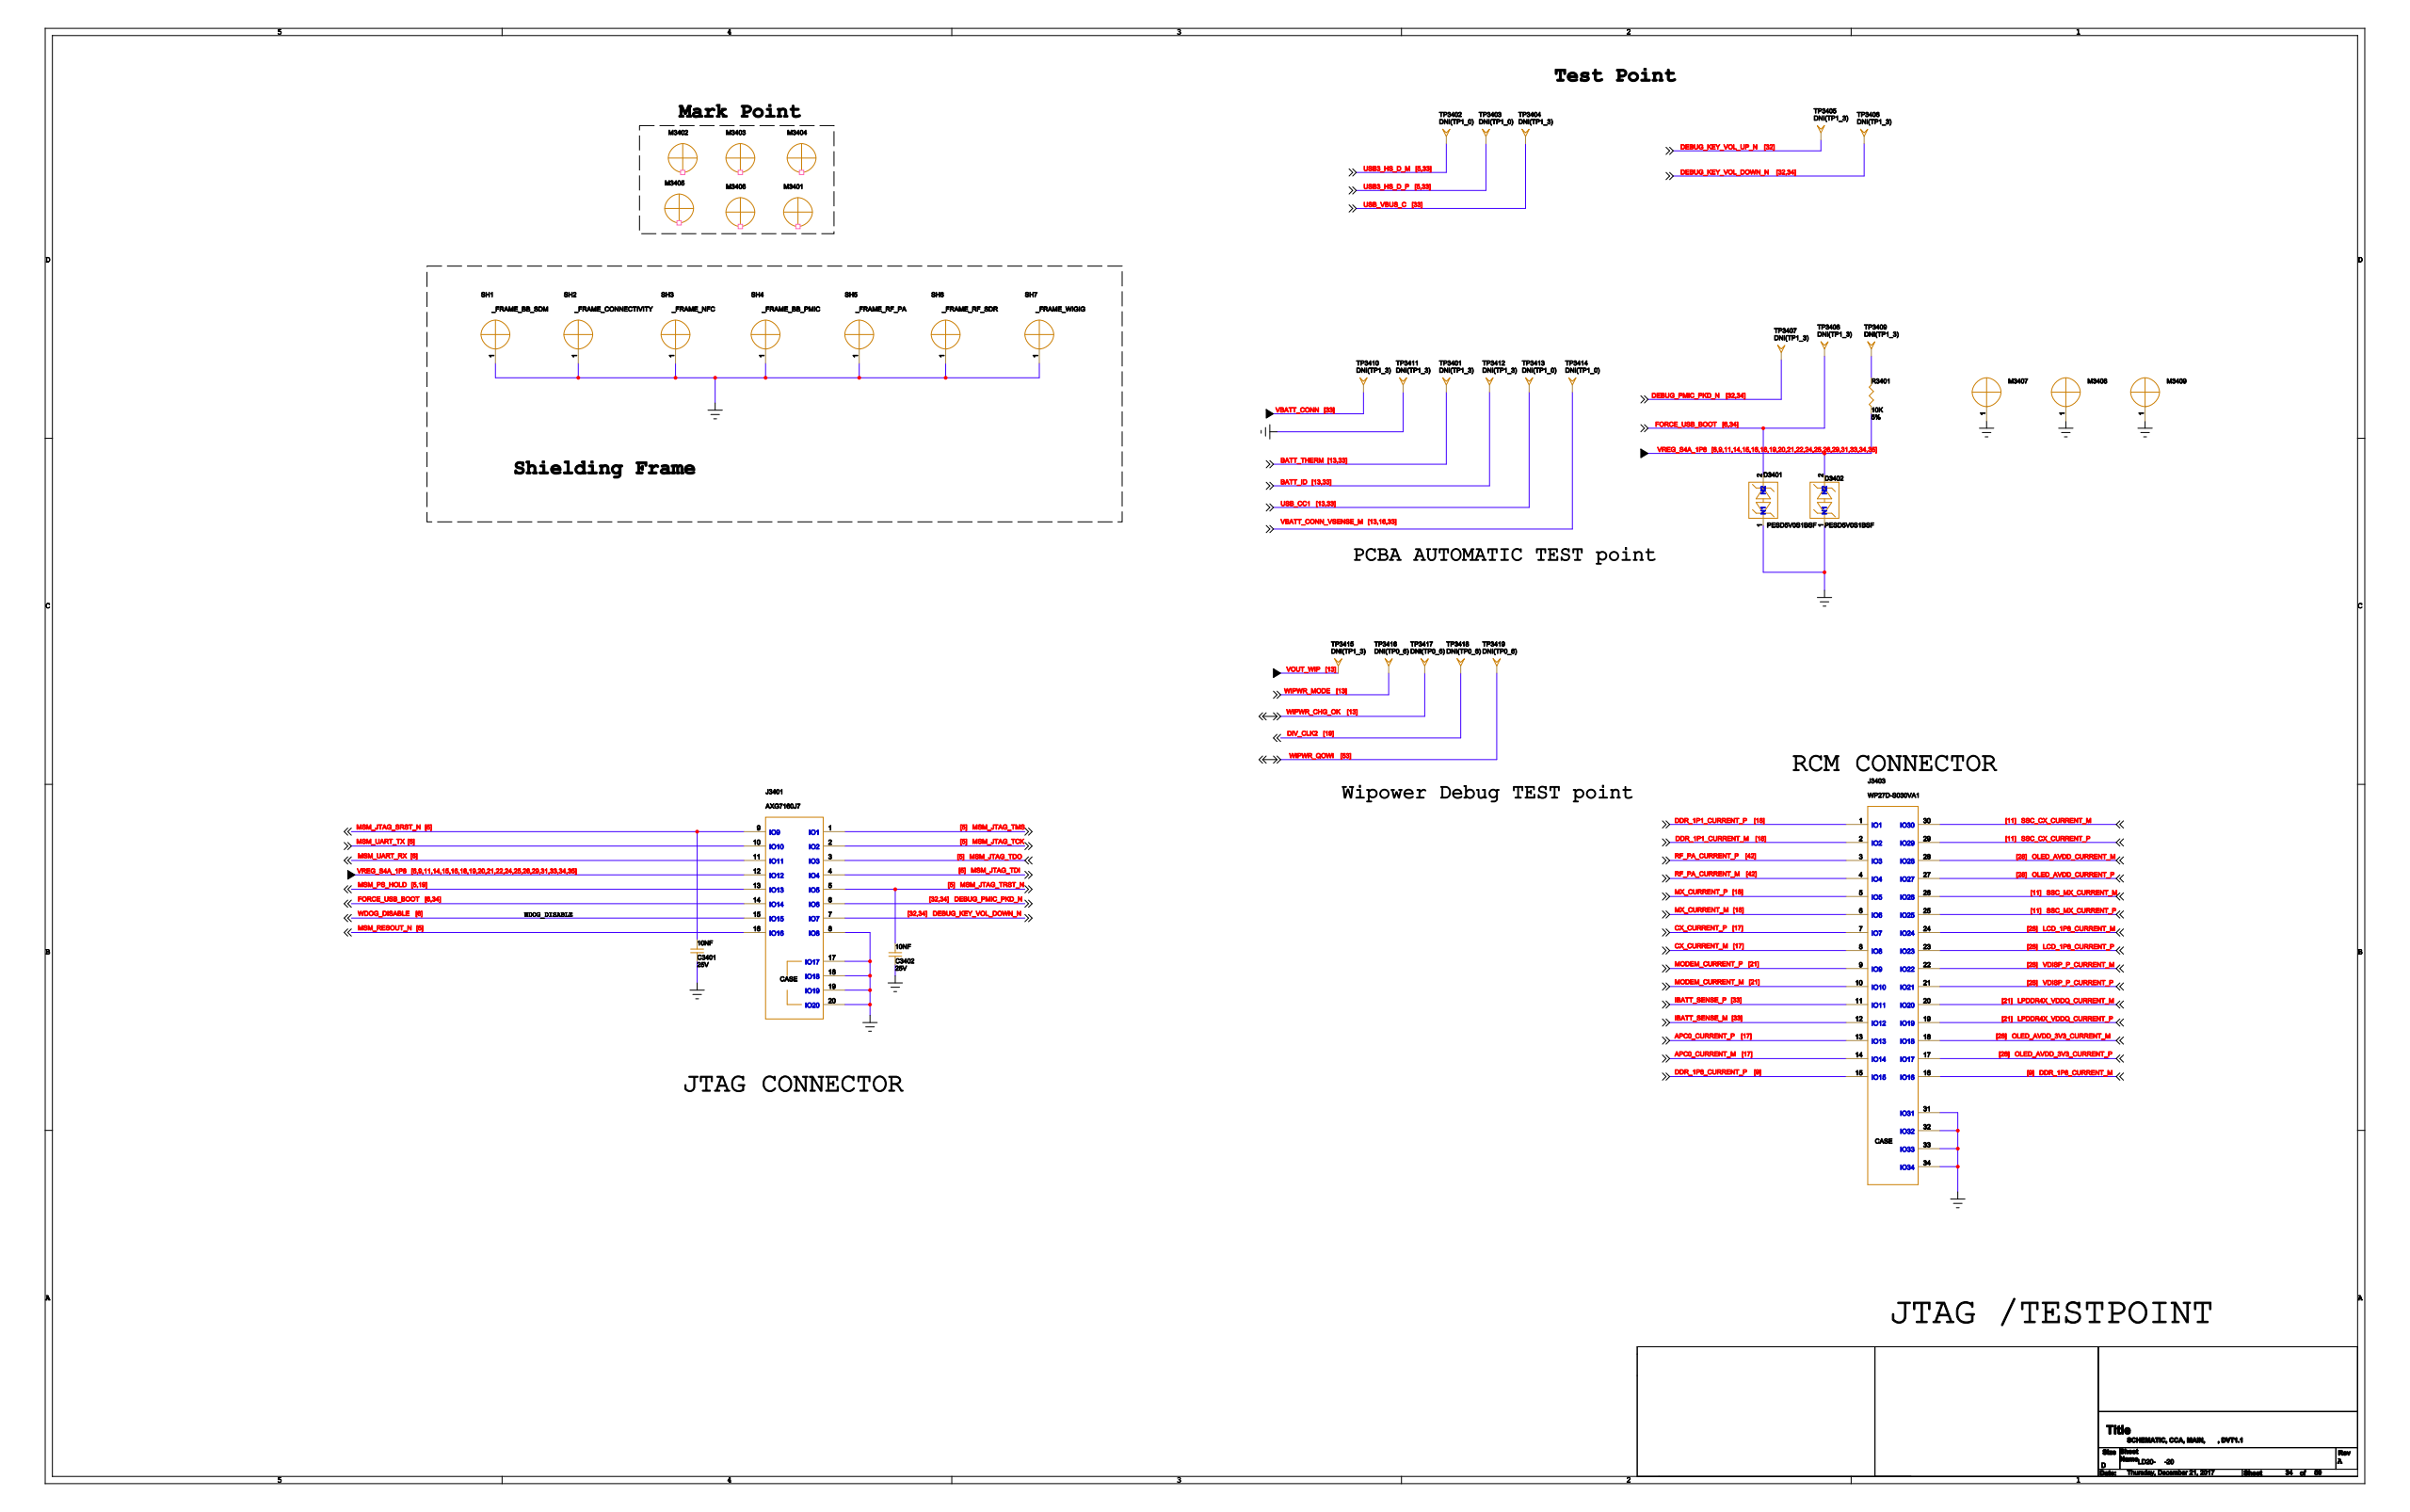Circuit board | Cadence Allegro | 1520 parts | 1149 nets | one sheet of the schematic
Parts on this sheet (reference | value | footprint):
C3401 | 10NF | 2P0402R
C3402 | 10NF | 2P0402R
D3401 | PESD5V0S1BSF | 2PSM25X13N
D3402 | PESD5V0S1BSF | 2PSM25X13N
J3401 | AXG7160J7 | 20SCONS138_CCW
J3403 | WP27D-S030VA1 | 34SCONS138V3_CCW
M3407 | DNI(PTH_HOLE) | PTH1_6
M3408 | DNI(PTH_HOLE) | PTH1_6
M3409 | DNI(PTH_HOLE) | PTH1_6
R3401 | 10K | 2P0201R
SH1 | xxxxxx_FRAME_BB_SDM | xxxxxx_FRAME_BB
SH2 | xxxxxx_FRAME_CONNECTIVITY | xxxxxx_FRAME_CONNECTIVITY
SH3 | xxxxxx_FRAME_NFC | xxxxxx_FRAME_NFC
SH4 | xxxxxx_FRAME_BB_PMIC | xxxxxx_FRAME_PMIC
SH5 | xxxxxx_FRAME_RF_PA | xxxxxx_FRAME_RFPA
SH6 | xxxxxx_FRAME_RF_SDR | xxxxxx_FRAME_SDR
SH7 | xxxxxx_FRAME_WIGIG | xxxxxx_FRAME_WIGIG
TP3401 | DNI(TP1_3) | TP-1_3
TP3402 | DNI(TP1_0) | TP-1_0
TP3403 | DNI(TP1_0) | TP-1_0
TP3404 | DNI(TP1_3) | TP-1_3
TP3405 | DNI(TP1_3) | TP-1_3
TP3406 | DNI(TP1_3) | TP-1_3
TP3407 | DNI(TP1_3) | TP-1_3
TP3408 | DNI(TP1_3) | TP-1_3
TP3409 | DNI(TP1_3) | TP-1_3
TP3410 | DNI(TP1_3) | TP-1_3
TP3411 | DNI(TP1_3) | TP-1_3
TP3412 | DNI(TP1_3) | TP-1_3
TP3413 | DNI(TP1_0) | TP-1_0
TP3414 | DNI(TP1_0) | TP-1_0
TP3415 | DNI(TP1_3) | TP-1_3
TP3416 | DNI(TP0_6) | TP-0_6
TP3417 | DNI(TP0_6) | TP-0_6
TP3418 | DNI(TP0_6) | TP-0_6
TP3419 | DNI(TP0_6) | TP-0_6
Nets of these parts (net: part-pin ...):
GND: C3401-1 C3402-1 D3401-1 D3402-1 J3401-8 J3401-17 J3401-18 J3401-19 J3401-20 M3407-1 M3408-1 M3409-1 SH1-1 SH2-1 SH3-1 SH4-1 SH5-1 SH6-1 SH7-1 TP3411-1 J3403-31 J3403-32 J3403-33 J3403-34
VREG_S4A_1P8: D3402-2 J3401-12 R3401-2
DDR_1P8_CURRENT_M: J3403-16
DDR_1P8_CURRENT_P: J3403-15
SSC_CX_CURRENT_P: J3403-29
SSC_CX_CURRENT_M: J3403-30
SSC_MX_CURRENT_P: J3403-25
SSC_MX_CURRENT_M: J3403-26
APC0_CURRENT_P: J3403-13
APC0_CURRENT_M: J3403-14
MX_CURRENT_P: J3403-5
MX_CURRENT_M: J3403-6
CX_CURRENT_P: J3403-7
CX_CURRENT_M: J3403-8
DDR_1P1_CURRENT_P: J3403-1
DDR_1P1_CURRENT_M: J3403-2
MODEM_CURRENT_P: J3403-9
MODEM_CURRENT_M: J3403-10
LPDDR4X_VDDQ_CURRENT_P: J3403-19
LPDDR4X_VDDQ_CURRENT_M: J3403-20
VDISP_P_CURRENT_P: J3403-21
VDISP_P_CURRENT_M: J3403-22
LCD_1P8_CURRENT_M: J3403-24
LCD_1P8_CURRENT_P: J3403-23
OLED_AVDD_CURRENT_M: J3403-28
OLED_AVDD_CURRENT_P: J3403-27
OLED_AVDD_3V3_CURRENT_M: J3403-18
OLED_AVDD_3V3_CURRENT_P: J3403-17
IBATT_SENSE_P: J3403-11
VBATT_CONN: TP3410-1
IBATT_SENSE_M: J3403-12
RF_PA_CURRENT_P: J3403-3
RF_PA_CURRENT_M: J3403-4
DEBUG_KEY_VOL_DOWN_N: J3401-7 TP3406-1
DEBUG_PMIC_PKD_N: J3401-6 TP3407-1
DEBUG_KEY_VOL_UP_N: TP3405-1
BATT_THERM: TP3401-1
BATT_ID: TP3412-1
VBATT_CONN_VSENSE_M: TP3414-1
FORCE_USB_BOOT: D3401-2 J3401-14 TP3408-1
VOUT_WIP: TP3415-1
USB_CC1: TP3413-1
MSM_JTAG_SRST_N: C3401-2 J3401-9
MSM_JTAG_TRST_N: C3402-2 J3401-5
WIPWR_MODE: TP3416-1
WIPWR_CHG_OK: TP3417-1
USB3_HS_D_M: TP3402-1
USB3_HS_D_P: TP3403-1
USB_VBUS_C: TP3404-1
MSM_JTAG_TMS: J3401-1
MSM_UART_TX: J3401-10
MSM_UART_RX: J3401-11
MSM_PS_HOLD: J3401-13
WDOG_DISABLE: J3401-15
MSM_RESOUT_N: J3401-16
MSM_JTAG_TCK: J3401-2
MSM_JTAG_TDO: J3401-3
MSM_JTAG_TDI: J3401-4
N24236066: R3401-1 TP3409-1
WIPWR_QOWI: TP3419-1
DIV_CLK2: TP3418-1